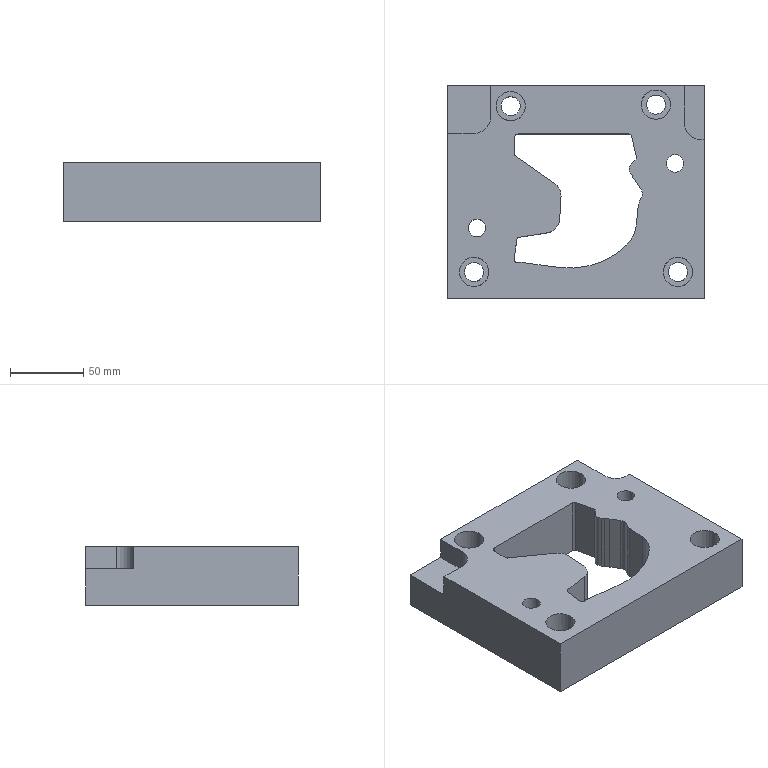Part | STEP file | gslz 2016.10.28-13_id178_x_t | 1 solid | 58 faces | box 175 x 145 x 40 mm | volume 717336 mm3 | plane 32 | cylinder 26 | commonest cylinder face diameters 20 x7 4 x5 13 x4 10 x2 12 x2 2 x1